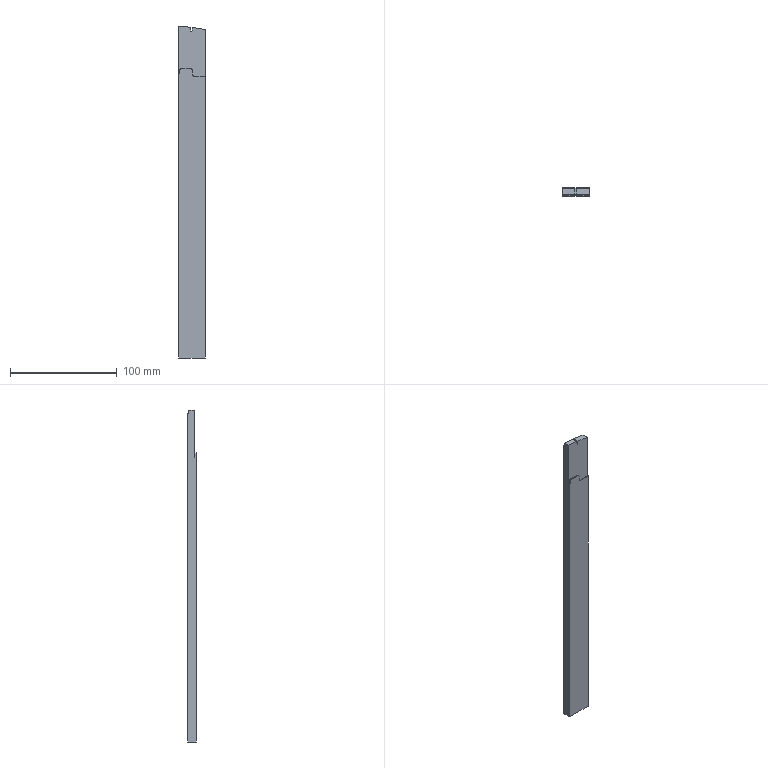Part | STEP file | P011002L004-000 | 1 solid | 91 faces | box 25 x 7.502 x 311.018 mm | volume 56283 mm3 | plane 52 | cylinder 10 | cone 10 | other 10 | spline 9 | commonest cylinder face diameters 4.048 x4 4.167 x2 4.983 x2 5 x2